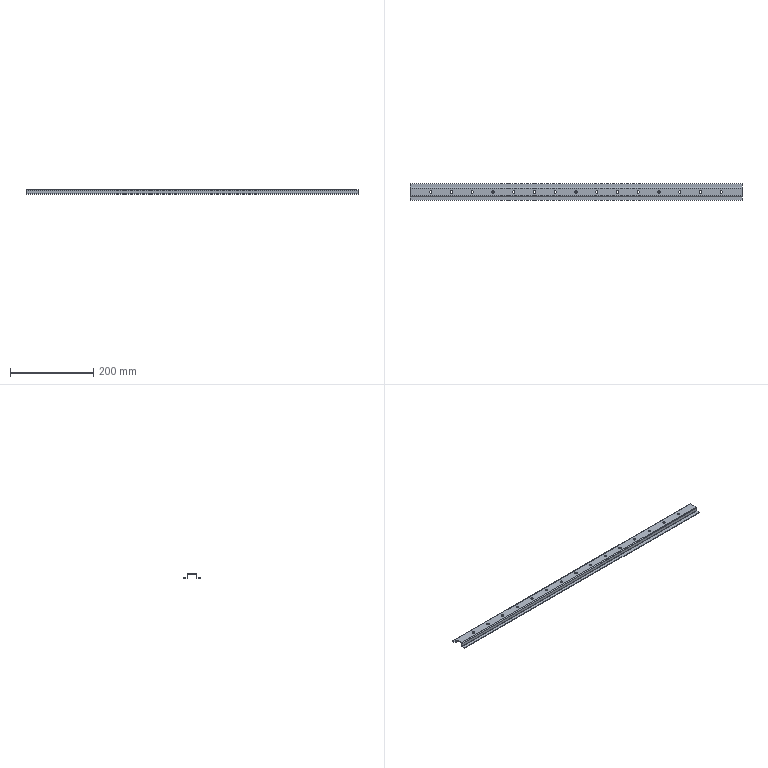Part | SolidWorks | features BaseBody 1 | 1 solid | 68 faces | box 800 x 40 x 11.5 mm | volume 68789 mm3 | cylinder 38 | plane 30 | commonest cylinder face diameters 6 x30 1 x4 4 x4